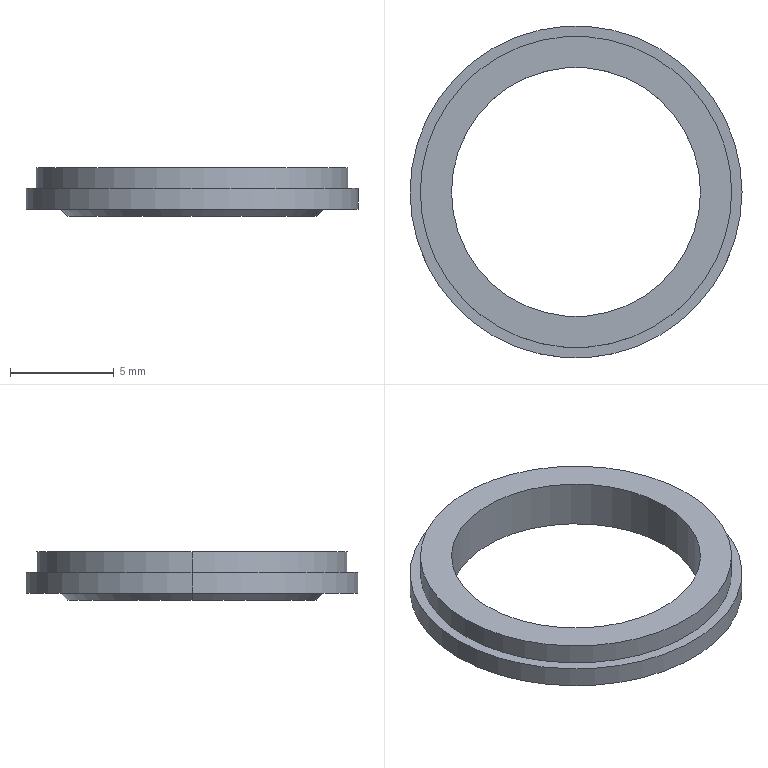Part | SolidWorks | features BaseBody 1 | 1 solid | 11 faces | box 16 x 16 x 2.338 mm | volume 153.776 mm3 | cylinder 6 | plane 3 | cone 2 | commonest cylinder face diameters 12 x2 15 x2 16 x2
STEP:
#1=CARTESIAN_POINT('',(572.22,76.38,31.475));
#2=VERTEX_POINT('',#1);
#3=CARTESIAN_POINT('',(560.22,76.38,31.475));
#4=VERTEX_POINT('',#3);
#5=CARTESIAN_POINT('',(566.22,76.38,31.475));
#6=DIRECTION('',(0.,0.,1.));
#7=DIRECTION('',(0.809,0.5878,0.));
#8=AXIS2_PLACEMENT_3D('',#5,#6,#7);
#9=CIRCLE('',#8,6.);
#10=EDGE_CURVE('',#2,#4,#9,.T.);
#11=ORIENTED_EDGE('',*,*,#10,.T.);
#12=CARTESIAN_POINT('',(559.882,76.38,31.813));
#13=VERTEX_POINT('',#12);
#14=CARTESIAN_POINT('',(559.882,76.38,31.813));
#15=DIRECTION('',(-0.7071,0.,0.7071));
#16=VECTOR('',#15,1000.);
#17=LINE('',#14,#16);
#18=EDGE_CURVE('',#4,#13,#17,.T.);
#19=ORIENTED_EDGE('',*,*,#18,.T.);
#20=CARTESIAN_POINT('',(572.558,76.38,31.813));
#21=VERTEX_POINT('',#20);
#22=CARTESIAN_POINT('',(566.22,76.38,31.813));
#23=DIRECTION('',(0.,0.,-1.));
#24=DIRECTION('',(1.,0.,0.));
#25=AXIS2_PLACEMENT_3D('',#22,#23,#24);
#26=CIRCLE('',#25,6.338);
#27=EDGE_CURVE('',#13,#21,#26,.T.);
#28=ORIENTED_EDGE('',*,*,#27,.T.);
#29=CARTESIAN_POINT('',(572.558,76.38,31.813));
#30=DIRECTION('',(0.7071,0.,0.7071));
#31=VECTOR('',#30,1000.);
#32=LINE('',#29,#31);
#33=EDGE_CURVE('',#2,#21,#32,.T.);
#34=ORIENTED_EDGE('',*,*,#33,.F.);
#35=EDGE_LOOP('',(#11,#19,#28,#34));
#36=FACE_OUTER_BOUND('',#35,.T.);
#37=CARTESIAN_POINT('',(566.22,76.38,31.813));
#38=DIRECTION('',(0.,0.,1.));
#39=DIRECTION('',(1.,0.,0.));
#40=AXIS2_PLACEMENT_3D('',#37,#38,#39);
#41=CONICAL_SURFACE('',#40,6.338,0.7854);
#42=ADVANCED_FACE('',(#36),#41,.T.);
#43=CARTESIAN_POINT('',(558.22,76.38,32.813));
#44=VERTEX_POINT('',#43);
#45=CARTESIAN_POINT('',(574.22,76.38,32.813));
#46=VERTEX_POINT('',#45);
#47=CARTESIAN_POINT('',(566.22,76.38,32.813));
#48=DIRECTION('',(0.,0.,-1.));
#49=DIRECTION('',(-1.,0.,0.));
#50=AXIS2_PLACEMENT_3D('',#47,#48,#49);
#51=CIRCLE('',#50,8.);
#52=EDGE_CURVE('',#44,#46,#51,.T.);
#53=ORIENTED_EDGE('',*,*,#52,.T.);
#54=CARTESIAN_POINT('',(574.22,76.38,31.813));
#55=VERTEX_POINT('',#54);
#56=CARTESIAN_POINT('',(574.22,76.38,32.313));
#57=DIRECTION('',(0.,0.,-1.));
#58=VECTOR('',#57,1000.);
#59=LINE('',#56,#58);
#60=EDGE_CURVE('',#46,#55,#59,.T.);
#61=ORIENTED_EDGE('',*,*,#60,.T.);
#62=CARTESIAN_POINT('',(558.22,76.38,31.813));
#63=VERTEX_POINT('',#62);
#64=CARTESIAN_POINT('',(566.22,76.38,31.813));
#65=DIRECTION('',(0.,0.,1.));
#66=DIRECTION('',(-1.,0.,0.));
#67=AXIS2_PLACEMENT_3D('',#64,#65,#66);
#68=CIRCLE('',#67,8.);
#69=EDGE_CURVE('',#55,#63,#68,.T.);
#70=ORIENTED_EDGE('',*,*,#69,.T.);
#71=CARTESIAN_POINT('',(558.22,76.38,32.313));
#72=DIRECTION('',(0.,0.,-1.));
#73=VECTOR('',#72,1000.);
#74=LINE('',#71,#73);
#75=EDGE_CURVE('',#44,#63,#74,.T.);
#76=ORIENTED_EDGE('',*,*,#75,.F.);
#77=EDGE_LOOP('',(#53,#61,#70,#76));
#78=FACE_OUTER_BOUND('',#77,.T.);
#79=CARTESIAN_POINT('',(566.22,76.38,32.313));
#80=DIRECTION('',(0.,0.,-1.));
#81=DIRECTION('',(-1.,0.,0.));
#82=AXIS2_PLACEMENT_3D('',#79,#80,#81);
#83=CYLINDRICAL_SURFACE('',#82,8.);
#84=ADVANCED_FACE('',(#78),#83,.T.);
#85=CARTESIAN_POINT('',(572.22,76.38,33.813));
#86=VERTEX_POINT('',#85);
#87=CARTESIAN_POINT('',(560.22,76.38,33.813));
#88=VERTEX_POINT('',#87);
#89=CARTESIAN_POINT('',(566.22,76.38,33.813));
#90=DIRECTION('',(0.,0.,-1.));
#91=DIRECTION('',(-1.,0.,0.));
#92=AXIS2_PLACEMENT_3D('',#89,#90,#91);
#93=CIRCLE('',#92,6.);
#94=EDGE_CURVE('',#86,#88,#93,.T.);
#95=ORIENTED_EDGE('',*,*,#94,.F.);
#96=CARTESIAN_POINT('',(572.22,76.38,41.813));
#97=DIRECTION('',(0.,0.,-1.));
#98=VECTOR('',#97,1000.);
#99=LINE('',#96,#98);
#100=EDGE_CURVE('',#86,#2,#99,.T.);
#101=ORIENTED_EDGE('',*,*,#100,.T.);
#102=CARTESIAN_POINT('',(566.22,76.38,31.475));
#103=DIRECTION('',(0.,0.,1.));
#104=DIRECTION('',(0.809,0.5878,0.));
#105=AXIS2_PLACEMENT_3D('',#102,#103,#104);
#106=CIRCLE('',#105,6.);
#107=EDGE_CURVE('',#4,#2,#106,.T.);
#108=ORIENTED_EDGE('',*,*,#107,.F.);
#109=CARTESIAN_POINT('',(560.22,76.38,41.813));
#110=DIRECTION('',(0.,0.,-1.));
#111=VECTOR('',#110,1000.);
#112=LINE('',#109,#111);
#113=EDGE_CURVE('',#88,#4,#112,.T.);
#114=ORIENTED_EDGE('',*,*,#113,.F.);
#115=EDGE_LOOP('',(#95,#101,#108,#114));
#116=FACE_OUTER_BOUND('',#115,.T.);
#117=CARTESIAN_POINT('',(566.22,76.38,41.813));
#118=DIRECTION('',(0.,0.,-1.));
#119=DIRECTION('',(-1.,0.,0.));
#120=AXIS2_PLACEMENT_3D('',#117,#118,#119);
#121=CYLINDRICAL_SURFACE('',#120,6.);
#122=ADVANCED_FACE('',(#116),#121,.F.);
#123=CARTESIAN_POINT('',(573.72,76.38,32.813));
#124=VERTEX_POINT('',#123);
#125=CARTESIAN_POINT('',(558.72,76.38,32.813));
#126=VERTEX_POINT('',#125);
#127=CARTESIAN_POINT('',(566.22,76.38,32.813));
#128=DIRECTION('',(0.,0.,1.));
#129=DIRECTION('',(1.,0.,0.));
#130=AXIS2_PLACEMENT_3D('',#127,#128,#129);
#131=CIRCLE('',#130,7.5);
#132=EDGE_CURVE('',#124,#126,#131,.T.);
#133=ORIENTED_EDGE('',*,*,#132,.T.);
#134=CARTESIAN_POINT('',(558.72,76.38,33.813));
#135=VERTEX_POINT('',#134);
#136=CARTESIAN_POINT('',(558.72,76.38,33.313));
#137=DIRECTION('',(0.,0.,1.));
#138=VECTOR('',#137,1000.);
#139=LINE('',#136,#138);
#140=EDGE_CURVE('',#126,#135,#139,.T.);
#141=ORIENTED_EDGE('',*,*,#140,.T.);
#142=CARTESIAN_POINT('',(573.72,76.38,33.813));
#143=VERTEX_POINT('',#142);
#144=CARTESIAN_POINT('',(566.22,76.38,33.813));
#145=DIRECTION('',(0.,0.,-1.));
#146=DIRECTION('',(1.,0.,0.));
#147=AXIS2_PLACEMENT_3D('',#144,#145,#146);
#148=CIRCLE('',#147,7.5);
#149=EDGE_CURVE('',#135,#143,#148,.T.);
#150=ORIENTED_EDGE('',*,*,#149,.T.);
#151=CARTESIAN_POINT('',(573.72,76.38,33.313));
#152=DIRECTION('',(0.,0.,1.));
#153=VECTOR('',#152,1000.);
#154=LINE('',#151,#153);
#155=EDGE_CURVE('',#124,#143,#154,.T.);
#156=ORIENTED_EDGE('',*,*,#155,.F.);
#157=EDGE_LOOP('',(#133,#141,#150,#156));
#158=FACE_OUTER_BOUND('',#157,.T.);
#159=CARTESIAN_POINT('',(566.22,76.38,33.313));
#160=DIRECTION('',(0.,0.,1.));
#161=DIRECTION('',(1.,0.,0.));
#162=AXIS2_PLACEMENT_3D('',#159,#160,#161);
#163=CYLINDRICAL_SURFACE('',#162,7.5);
#164=ADVANCED_FACE('',(#158),#163,.T.);
#165=CARTESIAN_POINT('',(566.22,76.38,31.813));
#166=DIRECTION('',(0.,0.,-1.));
#167=DIRECTION('',(1.,0.,0.));
#168=AXIS2_PLACEMENT_3D('',#165,#166,#167);
#169=CIRCLE('',#168,6.338);
#170=EDGE_CURVE('',#21,#13,#169,.T.);
#171=ORIENTED_EDGE('',*,*,#170,.F.);
#172=ORIENTED_EDGE('',*,*,#27,.F.);
#173=EDGE_LOOP('',(#171,#172));
#174=FACE_BOUND('',#173,.T.);
#175=CARTESIAN_POINT('',(566.22,76.38,31.813));
#176=DIRECTION('',(0.,0.,1.));
#177=DIRECTION('',(-1.,0.,0.));
#178=AXIS2_PLACEMENT_3D('',#175,#176,#177);
#179=CIRCLE('',#178,8.);
#180=EDGE_CURVE('',#63,#55,#179,.T.);
#181=ORIENTED_EDGE('',*,*,#180,.F.);
#182=ORIENTED_EDGE('',*,*,#69,.F.);
#183=EDGE_LOOP('',(#181,#182));
#184=FACE_OUTER_BOUND('',#183,.T.);
#185=CARTESIAN_POINT('',(566.22,76.38,31.813));
#186=DIRECTION('',(0.,0.,1.));
#187=DIRECTION('',(1.,0.,0.));
#188=AXIS2_PLACEMENT_3D('',#185,#186,#187);
#189=PLANE('',#188);
#190=ADVANCED_FACE('',(#174,#184),#189,.F.);
#191=ORIENTED_EDGE('',*,*,#18,.F.);
#192=ORIENTED_EDGE('',*,*,#107,.T.);
#193=ORIENTED_EDGE('',*,*,#33,.T.);
#194=ORIENTED_EDGE('',*,*,#170,.T.);
#195=EDGE_LOOP('',(#191,#192,#193,#194));
#196=FACE_OUTER_BOUND('',#195,.T.);
#197=CARTESIAN_POINT('',(566.22,76.38,31.813));
#198=DIRECTION('',(0.,0.,1.));
#199=DIRECTION('',(1.,0.,0.));
#200=AXIS2_PLACEMENT_3D('',#197,#198,#199);
#201=CONICAL_SURFACE('',#200,6.338,0.7854);
#202=ADVANCED_FACE('',(#196),#201,.T.);
#203=ORIENTED_EDGE('',*,*,#60,.F.);
#204=CARTESIAN_POINT('',(566.22,76.38,32.813));
#205=DIRECTION('',(0.,0.,-1.));
#206=DIRECTION('',(-1.,0.,0.));
#207=AXIS2_PLACEMENT_3D('',#204,#205,#206);
#208=CIRCLE('',#207,8.);
#209=EDGE_CURVE('',#46,#44,#208,.T.);
#210=ORIENTED_EDGE('',*,*,#209,.T.);
#211=ORIENTED_EDGE('',*,*,#75,.T.);
#212=ORIENTED_EDGE('',*,*,#180,.T.);
#213=EDGE_LOOP('',(#203,#210,#211,#212));
#214=FACE_OUTER_BOUND('',#213,.T.);
#215=CARTESIAN_POINT('',(566.22,76.38,32.313));
#216=DIRECTION('',(0.,0.,-1.));
#217=DIRECTION('',(-1.,0.,0.));
#218=AXIS2_PLACEMENT_3D('',#215,#216,#217);
#219=CYLINDRICAL_SURFACE('',#218,8.);
#220=ADVANCED_FACE('',(#214),#219,.T.);
#221=ORIENTED_EDGE('',*,*,#100,.F.);
#222=CARTESIAN_POINT('',(566.22,76.38,33.813));
#223=DIRECTION('',(0.,0.,-1.));
#224=DIRECTION('',(-1.,0.,0.));
#225=AXIS2_PLACEMENT_3D('',#222,#223,#224);
#226=CIRCLE('',#225,6.);
#227=EDGE_CURVE('',#88,#86,#226,.T.);
#228=ORIENTED_EDGE('',*,*,#227,.F.);
#229=ORIENTED_EDGE('',*,*,#113,.T.);
#230=ORIENTED_EDGE('',*,*,#10,.F.);
#231=EDGE_LOOP('',(#221,#228,#229,#230));
#232=FACE_OUTER_BOUND('',#231,.T.);
#233=CARTESIAN_POINT('',(566.22,76.38,41.813));
#234=DIRECTION('',(0.,0.,-1.));
#235=DIRECTION('',(-1.,0.,0.));
#236=AXIS2_PLACEMENT_3D('',#233,#234,#235);
#237=CYLINDRICAL_SURFACE('',#236,6.);
#238=ADVANCED_FACE('',(#232),#237,.F.);
#239=ORIENTED_EDGE('',*,*,#132,.F.);
#240=CARTESIAN_POINT('',(566.22,76.38,32.813));
#241=DIRECTION('',(0.,0.,1.));
#242=DIRECTION('',(1.,0.,0.));
#243=AXIS2_PLACEMENT_3D('',#240,#241,#242);
#244=CIRCLE('',#243,7.5);
#245=EDGE_CURVE('',#126,#124,#244,.T.);
#246=ORIENTED_EDGE('',*,*,#245,.F.);
#247=EDGE_LOOP('',(#239,#246));
#248=FACE_BOUND('',#247,.T.);
#249=ORIENTED_EDGE('',*,*,#52,.F.);
#250=ORIENTED_EDGE('',*,*,#209,.F.);
#251=EDGE_LOOP('',(#249,#250));
#252=FACE_OUTER_BOUND('',#251,.T.);
#253=CARTESIAN_POINT('',(562.106,86.312,32.813));
#254=DIRECTION('',(0.,0.,-1.));
#255=DIRECTION('',(-1.,0.,0.));
#256=AXIS2_PLACEMENT_3D('',#253,#254,#255);
#257=PLANE('',#256);
#258=ADVANCED_FACE('',(#248,#252),#257,.F.);
#259=ORIENTED_EDGE('',*,*,#227,.T.);
#260=ORIENTED_EDGE('',*,*,#94,.T.);
#261=EDGE_LOOP('',(#259,#260));
#262=FACE_BOUND('',#261,.T.);
#263=CARTESIAN_POINT('',(566.22,76.38,33.813));
#264=DIRECTION('',(0.,0.,-1.));
#265=DIRECTION('',(1.,0.,0.));
#266=AXIS2_PLACEMENT_3D('',#263,#264,#265);
#267=CIRCLE('',#266,7.5);
#268=EDGE_CURVE('',#143,#135,#267,.T.);
#269=ORIENTED_EDGE('',*,*,#268,.F.);
#270=ORIENTED_EDGE('',*,*,#149,.F.);
#271=EDGE_LOOP('',(#269,#270));
#272=FACE_OUTER_BOUND('',#271,.T.);
#273=CARTESIAN_POINT('',(564.785,79.845,33.813));
#274=DIRECTION('',(0.,0.,-1.));
#275=DIRECTION('',(-1.,0.,0.));
#276=AXIS2_PLACEMENT_3D('',#273,#274,#275);
#277=PLANE('',#276);
#278=ADVANCED_FACE('',(#262,#272),#277,.F.);
#279=ORIENTED_EDGE('',*,*,#140,.F.);
#280=ORIENTED_EDGE('',*,*,#245,.T.);
#281=ORIENTED_EDGE('',*,*,#155,.T.);
#282=ORIENTED_EDGE('',*,*,#268,.T.);
#283=EDGE_LOOP('',(#279,#280,#281,#282));
#284=FACE_OUTER_BOUND('',#283,.T.);
#285=CARTESIAN_POINT('',(566.22,76.38,33.313));
#286=DIRECTION('',(0.,0.,1.));
#287=DIRECTION('',(1.,0.,0.));
#288=AXIS2_PLACEMENT_3D('',#285,#286,#287);
#289=CYLINDRICAL_SURFACE('',#288,7.5);
#290=ADVANCED_FACE('',(#284),#289,.T.);
#291=CLOSED_SHELL('',(#42,#84,#122,#164,#190,#202,#220,#238,#258,#278,#290));
#292=MANIFOLD_SOLID_BREP('',#291);
#293=CARTESIAN_POINT('',(0.,0.,0.));
#294=DIRECTION('',(0.,0.,1.));
#295=DIRECTION('',(1.,0.,0.));
#296=AXIS2_PLACEMENT_3D('',#293,#294,#295);
#297=(LENGTH_UNIT()NAMED_UNIT(*)SI_UNIT(.MILLI.,.METRE.));
#298=UNCERTAINTY_MEASURE_WITH_UNIT(LENGTH_MEASURE(0.00001),#297,'','');
#299=(NAMED_UNIT(*)PLANE_ANGLE_UNIT()SI_UNIT($,.RADIAN.));
#300=(NAMED_UNIT(*)SI_UNIT($,.STERADIAN.)SOLID_ANGLE_UNIT());
#301=(GEOMETRIC_REPRESENTATION_CONTEXT(3)GLOBAL_UNCERTAINTY_ASSIGNED_CONTEXT((#298))GLOBAL_UNIT_ASSIGNED_CONTEXT((#297,#299,#300))REPRESENTATION_CONTEXT('',''));
#302=ADVANCED_BREP_SHAPE_REPRESENTATION('',(#292,#296),#301);